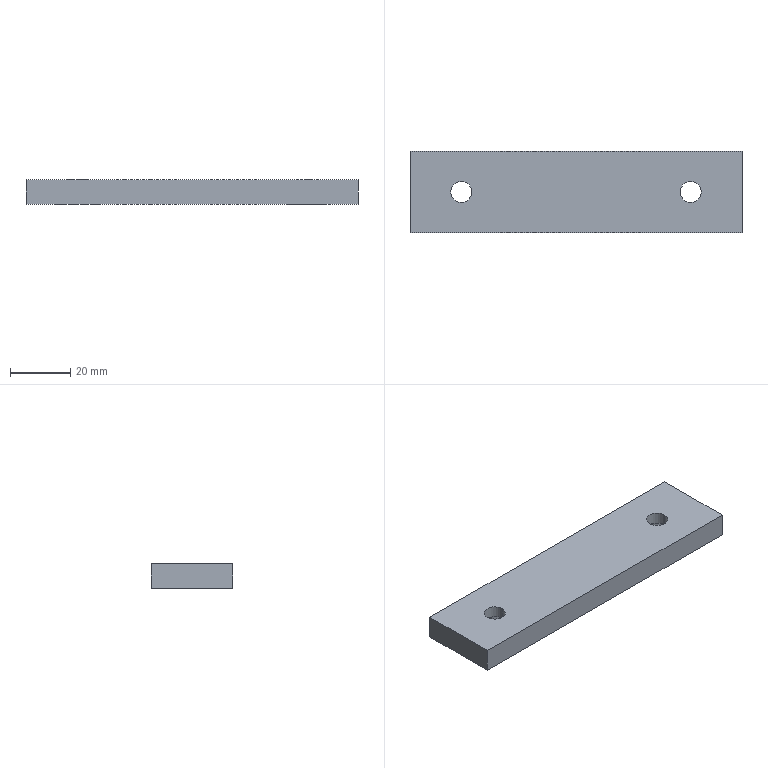Part | SolidWorks | features Extrusion 1, MirrorPattern 1, RevCut 1 | 1 solid | 14 faces | box 110 x 27 x 8 mm | volume 22658 mm3 | plane 6 | cylinder 4 | cone 4 | commonest cylinder face diameters 7 x4
STEP:
#1=CARTESIAN_POINT('',(41.5,0.,8.));
#2=VERTEX_POINT('',#1);
#3=CARTESIAN_POINT('',(34.5,0.,8.));
#4=VERTEX_POINT('',#3);
#5=CARTESIAN_POINT('',(38.,0.,8.));
#6=DIRECTION('',(0.,0.,1.));
#7=DIRECTION('',(1.,0.,0.));
#8=AXIS2_PLACEMENT_3D('',#5,#6,#7);
#9=CIRCLE('',#8,3.5);
#10=EDGE_CURVE('',#2,#4,#9,.T.);
#11=ORIENTED_EDGE('',*,*,#10,.T.);
#12=CARTESIAN_POINT('',(34.5,0.,4.));
#13=VERTEX_POINT('',#12);
#14=CARTESIAN_POINT('',(34.5,0.,0.));
#15=DIRECTION('',(0.,0.,-1.));
#16=VECTOR('',#15,1000.);
#17=LINE('',#14,#16);
#18=EDGE_CURVE('',#4,#13,#17,.T.);
#19=ORIENTED_EDGE('',*,*,#18,.T.);
#20=CARTESIAN_POINT('',(41.5,0.,4.));
#21=VERTEX_POINT('',#20);
#22=CARTESIAN_POINT('',(38.,0.,4.));
#23=DIRECTION('',(0.,0.,1.));
#24=DIRECTION('',(1.,0.,0.));
#25=AXIS2_PLACEMENT_3D('',#22,#23,#24);
#26=CIRCLE('',#25,3.5);
#27=EDGE_CURVE('',#21,#13,#26,.T.);
#28=ORIENTED_EDGE('',*,*,#27,.F.);
#29=CARTESIAN_POINT('',(41.5,0.,0.));
#30=DIRECTION('',(0.,0.,-1.));
#31=VECTOR('',#30,1000.);
#32=LINE('',#29,#31);
#33=EDGE_CURVE('',#2,#21,#32,.T.);
#34=ORIENTED_EDGE('',*,*,#33,.F.);
#35=EDGE_LOOP('',(#11,#19,#28,#34));
#36=FACE_OUTER_BOUND('',#35,.T.);
#37=CARTESIAN_POINT('',(38.,0.,0.));
#38=DIRECTION('',(0.,0.,-1.));
#39=DIRECTION('',(1.,0.,0.));
#40=AXIS2_PLACEMENT_3D('',#37,#38,#39);
#41=CYLINDRICAL_SURFACE('',#40,3.5);
#42=ADVANCED_FACE('',(#36),#41,.F.);
#43=ORIENTED_EDGE('',*,*,#27,.T.);
#44=CARTESIAN_POINT('',(30.5,0.,0.));
#45=VERTEX_POINT('',#44);
#46=CARTESIAN_POINT('',(34.5,0.,4.));
#47=DIRECTION('',(-0.7071,0.,-0.7071));
#48=VECTOR('',#47,1000.);
#49=LINE('',#46,#48);
#50=EDGE_CURVE('',#13,#45,#49,.T.);
#51=ORIENTED_EDGE('',*,*,#50,.T.);
#52=CARTESIAN_POINT('',(45.5,0.,0.));
#53=VERTEX_POINT('',#52);
#54=CARTESIAN_POINT('',(38.,0.,0.));
#55=DIRECTION('',(0.,0.,1.));
#56=DIRECTION('',(1.,0.,0.));
#57=AXIS2_PLACEMENT_3D('',#54,#55,#56);
#58=CIRCLE('',#57,7.5);
#59=EDGE_CURVE('',#53,#45,#58,.T.);
#60=ORIENTED_EDGE('',*,*,#59,.F.);
#61=CARTESIAN_POINT('',(41.5,0.,4.));
#62=DIRECTION('',(0.7071,0.,-0.7071));
#63=VECTOR('',#62,1000.);
#64=LINE('',#61,#63);
#65=EDGE_CURVE('',#21,#53,#64,.T.);
#66=ORIENTED_EDGE('',*,*,#65,.F.);
#67=EDGE_LOOP('',(#43,#51,#60,#66));
#68=FACE_OUTER_BOUND('',#67,.T.);
#69=CARTESIAN_POINT('',(38.,0.,4.));
#70=DIRECTION('',(0.,0.,-1.));
#71=DIRECTION('',(1.,0.,0.));
#72=AXIS2_PLACEMENT_3D('',#69,#70,#71);
#73=CONICAL_SURFACE('',#72,3.5,0.7854);
#74=ADVANCED_FACE('',(#68),#73,.F.);
#75=CARTESIAN_POINT('',(-34.5,0.,8.));
#76=VERTEX_POINT('',#75);
#77=CARTESIAN_POINT('',(-41.5,0.,8.));
#78=VERTEX_POINT('',#77);
#79=CARTESIAN_POINT('',(-38.,0.,8.));
#80=DIRECTION('',(0.,0.,-1.));
#81=DIRECTION('',(-1.,0.,0.));
#82=AXIS2_PLACEMENT_3D('',#79,#80,#81);
#83=CIRCLE('',#82,3.5);
#84=EDGE_CURVE('',#76,#78,#83,.T.);
#85=ORIENTED_EDGE('',*,*,#84,.F.);
#86=CARTESIAN_POINT('',(-34.5,0.,4.));
#87=VERTEX_POINT('',#86);
#88=CARTESIAN_POINT('',(-34.5,0.,0.));
#89=DIRECTION('',(0.,0.,-1.));
#90=VECTOR('',#89,1000.);
#91=LINE('',#88,#90);
#92=EDGE_CURVE('',#76,#87,#91,.T.);
#93=ORIENTED_EDGE('',*,*,#92,.T.);
#94=CARTESIAN_POINT('',(-41.5,0.,4.));
#95=VERTEX_POINT('',#94);
#96=CARTESIAN_POINT('',(-38.,0.,4.));
#97=DIRECTION('',(0.,0.,-1.));
#98=DIRECTION('',(-1.,0.,0.));
#99=AXIS2_PLACEMENT_3D('',#96,#97,#98);
#100=CIRCLE('',#99,3.5);
#101=EDGE_CURVE('',#87,#95,#100,.T.);
#102=ORIENTED_EDGE('',*,*,#101,.T.);
#103=CARTESIAN_POINT('',(-41.5,0.,0.));
#104=DIRECTION('',(0.,0.,-1.));
#105=VECTOR('',#104,1000.);
#106=LINE('',#103,#105);
#107=EDGE_CURVE('',#78,#95,#106,.T.);
#108=ORIENTED_EDGE('',*,*,#107,.F.);
#109=EDGE_LOOP('',(#85,#93,#102,#108));
#110=FACE_OUTER_BOUND('',#109,.T.);
#111=CARTESIAN_POINT('',(-38.,0.,0.));
#112=DIRECTION('',(0.,0.,-1.));
#113=DIRECTION('',(-1.,0.,0.));
#114=AXIS2_PLACEMENT_3D('',#111,#112,#113);
#115=CYLINDRICAL_SURFACE('',#114,3.5);
#116=ADVANCED_FACE('',(#110),#115,.F.);
#117=ORIENTED_EDGE('',*,*,#101,.F.);
#118=CARTESIAN_POINT('',(-30.5,0.,0.));
#119=VERTEX_POINT('',#118);
#120=CARTESIAN_POINT('',(-34.5,0.,4.));
#121=DIRECTION('',(0.7071,0.,-0.7071));
#122=VECTOR('',#121,1000.);
#123=LINE('',#120,#122);
#124=EDGE_CURVE('',#87,#119,#123,.T.);
#125=ORIENTED_EDGE('',*,*,#124,.T.);
#126=CARTESIAN_POINT('',(-45.5,0.,0.));
#127=VERTEX_POINT('',#126);
#128=CARTESIAN_POINT('',(-38.,0.,0.));
#129=DIRECTION('',(0.,0.,-1.));
#130=DIRECTION('',(-1.,0.,0.));
#131=AXIS2_PLACEMENT_3D('',#128,#129,#130);
#132=CIRCLE('',#131,7.5);
#133=EDGE_CURVE('',#119,#127,#132,.T.);
#134=ORIENTED_EDGE('',*,*,#133,.T.);
#135=CARTESIAN_POINT('',(-41.5,0.,4.));
#136=DIRECTION('',(-0.7071,0.,-0.7071));
#137=VECTOR('',#136,1000.);
#138=LINE('',#135,#137);
#139=EDGE_CURVE('',#95,#127,#138,.T.);
#140=ORIENTED_EDGE('',*,*,#139,.F.);
#141=EDGE_LOOP('',(#117,#125,#134,#140));
#142=FACE_OUTER_BOUND('',#141,.T.);
#143=CARTESIAN_POINT('',(-38.,0.,4.));
#144=DIRECTION('',(0.,0.,-1.));
#145=DIRECTION('',(-1.,0.,0.));
#146=AXIS2_PLACEMENT_3D('',#143,#144,#145);
#147=CONICAL_SURFACE('',#146,3.5,0.7854);
#148=ADVANCED_FACE('',(#142),#147,.F.);
#149=CARTESIAN_POINT('',(55.,-13.5,0.));
#150=VERTEX_POINT('',#149);
#151=CARTESIAN_POINT('',(55.,13.5,0.));
#152=VERTEX_POINT('',#151);
#153=CARTESIAN_POINT('',(55.,-13.5,0.));
#154=DIRECTION('',(0.,1.,0.));
#155=VECTOR('',#154,1000.);
#156=LINE('',#153,#155);
#157=EDGE_CURVE('',#150,#152,#156,.T.);
#158=ORIENTED_EDGE('',*,*,#157,.T.);
#159=CARTESIAN_POINT('',(55.,13.5,8.));
#160=VERTEX_POINT('',#159);
#161=CARTESIAN_POINT('',(55.,13.5,8.));
#162=DIRECTION('',(0.,0.,-1.));
#163=VECTOR('',#162,1000.);
#164=LINE('',#161,#163);
#165=EDGE_CURVE('',#160,#152,#164,.T.);
#166=ORIENTED_EDGE('',*,*,#165,.F.);
#167=CARTESIAN_POINT('',(55.,-13.5,8.));
#168=VERTEX_POINT('',#167);
#169=CARTESIAN_POINT('',(55.,-13.5,8.));
#170=DIRECTION('',(0.,1.,0.));
#171=VECTOR('',#170,1000.);
#172=LINE('',#169,#171);
#173=EDGE_CURVE('',#168,#160,#172,.T.);
#174=ORIENTED_EDGE('',*,*,#173,.F.);
#175=CARTESIAN_POINT('',(55.,-13.5,8.));
#176=DIRECTION('',(0.,0.,-1.));
#177=VECTOR('',#176,1000.);
#178=LINE('',#175,#177);
#179=EDGE_CURVE('',#168,#150,#178,.T.);
#180=ORIENTED_EDGE('',*,*,#179,.T.);
#181=EDGE_LOOP('',(#158,#166,#174,#180));
#182=FACE_OUTER_BOUND('',#181,.T.);
#183=CARTESIAN_POINT('',(55.,-13.5,8.));
#184=DIRECTION('',(-1.,0.,0.));
#185=DIRECTION('',(0.,0.,1.));
#186=AXIS2_PLACEMENT_3D('',#183,#184,#185);
#187=PLANE('',#186);
#188=ADVANCED_FACE('',(#182),#187,.F.);
#189=CARTESIAN_POINT('',(-55.,13.5,0.));
#190=VERTEX_POINT('',#189);
#191=CARTESIAN_POINT('',(-55.,13.5,0.));
#192=DIRECTION('',(-1.,0.,0.));
#193=VECTOR('',#192,1000.);
#194=LINE('',#191,#193);
#195=EDGE_CURVE('',#152,#190,#194,.T.);
#196=ORIENTED_EDGE('',*,*,#195,.T.);
#197=CARTESIAN_POINT('',(-55.,13.5,8.));
#198=VERTEX_POINT('',#197);
#199=CARTESIAN_POINT('',(-55.,13.5,8.));
#200=DIRECTION('',(0.,0.,-1.));
#201=VECTOR('',#200,1000.);
#202=LINE('',#199,#201);
#203=EDGE_CURVE('',#198,#190,#202,.T.);
#204=ORIENTED_EDGE('',*,*,#203,.F.);
#205=CARTESIAN_POINT('',(-55.,13.5,8.));
#206=DIRECTION('',(-1.,0.,0.));
#207=VECTOR('',#206,1000.);
#208=LINE('',#205,#207);
#209=EDGE_CURVE('',#160,#198,#208,.T.);
#210=ORIENTED_EDGE('',*,*,#209,.F.);
#211=ORIENTED_EDGE('',*,*,#165,.T.);
#212=EDGE_LOOP('',(#196,#204,#210,#211));
#213=FACE_OUTER_BOUND('',#212,.T.);
#214=CARTESIAN_POINT('',(-55.,13.5,8.));
#215=DIRECTION('',(0.,-1.,0.));
#216=DIRECTION('',(0.,0.,-1.));
#217=AXIS2_PLACEMENT_3D('',#214,#215,#216);
#218=PLANE('',#217);
#219=ADVANCED_FACE('',(#213),#218,.F.);
#220=CARTESIAN_POINT('',(-55.,-13.5,0.));
#221=VERTEX_POINT('',#220);
#222=CARTESIAN_POINT('',(-55.,-13.5,0.));
#223=DIRECTION('',(0.,-1.,0.));
#224=VECTOR('',#223,1000.);
#225=LINE('',#222,#224);
#226=EDGE_CURVE('',#190,#221,#225,.T.);
#227=ORIENTED_EDGE('',*,*,#226,.T.);
#228=CARTESIAN_POINT('',(-55.,-13.5,8.));
#229=VERTEX_POINT('',#228);
#230=CARTESIAN_POINT('',(-55.,-13.5,8.));
#231=DIRECTION('',(0.,0.,-1.));
#232=VECTOR('',#231,1000.);
#233=LINE('',#230,#232);
#234=EDGE_CURVE('',#229,#221,#233,.T.);
#235=ORIENTED_EDGE('',*,*,#234,.F.);
#236=CARTESIAN_POINT('',(-55.,-13.5,8.));
#237=DIRECTION('',(0.,-1.,0.));
#238=VECTOR('',#237,1000.);
#239=LINE('',#236,#238);
#240=EDGE_CURVE('',#198,#229,#239,.T.);
#241=ORIENTED_EDGE('',*,*,#240,.F.);
#242=ORIENTED_EDGE('',*,*,#203,.T.);
#243=EDGE_LOOP('',(#227,#235,#241,#242));
#244=FACE_OUTER_BOUND('',#243,.T.);
#245=CARTESIAN_POINT('',(-55.,-13.5,8.));
#246=DIRECTION('',(1.,0.,0.));
#247=DIRECTION('',(0.,0.,-1.));
#248=AXIS2_PLACEMENT_3D('',#245,#246,#247);
#249=PLANE('',#248);
#250=ADVANCED_FACE('',(#244),#249,.F.);
#251=CARTESIAN_POINT('',(-55.,-13.5,0.));
#252=DIRECTION('',(1.,0.,0.));
#253=VECTOR('',#252,1000.);
#254=LINE('',#251,#253);
#255=EDGE_CURVE('',#221,#150,#254,.T.);
#256=ORIENTED_EDGE('',*,*,#255,.T.);
#257=ORIENTED_EDGE('',*,*,#179,.F.);
#258=CARTESIAN_POINT('',(-55.,-13.5,8.));
#259=DIRECTION('',(1.,0.,0.));
#260=VECTOR('',#259,1000.);
#261=LINE('',#258,#260);
#262=EDGE_CURVE('',#229,#168,#261,.T.);
#263=ORIENTED_EDGE('',*,*,#262,.F.);
#264=ORIENTED_EDGE('',*,*,#234,.T.);
#265=EDGE_LOOP('',(#256,#257,#263,#264));
#266=FACE_OUTER_BOUND('',#265,.T.);
#267=CARTESIAN_POINT('',(-55.,-13.5,8.));
#268=DIRECTION('',(0.,1.,0.));
#269=DIRECTION('',(0.,0.,1.));
#270=AXIS2_PLACEMENT_3D('',#267,#268,#269);
#271=PLANE('',#270);
#272=ADVANCED_FACE('',(#266),#271,.F.);
#273=ORIENTED_EDGE('',*,*,#10,.F.);
#274=CARTESIAN_POINT('',(38.,0.,8.));
#275=DIRECTION('',(0.,0.,1.));
#276=DIRECTION('',(1.,0.,0.));
#277=AXIS2_PLACEMENT_3D('',#274,#275,#276);
#278=CIRCLE('',#277,3.5);
#279=EDGE_CURVE('',#4,#2,#278,.T.);
#280=ORIENTED_EDGE('',*,*,#279,.F.);
#281=EDGE_LOOP('',(#273,#280));
#282=FACE_BOUND('',#281,.T.);
#283=CARTESIAN_POINT('',(-38.,0.,8.));
#284=DIRECTION('',(0.,0.,-1.));
#285=DIRECTION('',(-1.,0.,0.));
#286=AXIS2_PLACEMENT_3D('',#283,#284,#285);
#287=CIRCLE('',#286,3.5);
#288=EDGE_CURVE('',#78,#76,#287,.T.);
#289=ORIENTED_EDGE('',*,*,#288,.T.);
#290=ORIENTED_EDGE('',*,*,#84,.T.);
#291=EDGE_LOOP('',(#289,#290));
#292=FACE_BOUND('',#291,.T.);
#293=ORIENTED_EDGE('',*,*,#173,.T.);
#294=ORIENTED_EDGE('',*,*,#209,.T.);
#295=ORIENTED_EDGE('',*,*,#240,.T.);
#296=ORIENTED_EDGE('',*,*,#262,.T.);
#297=EDGE_LOOP('',(#293,#294,#295,#296));
#298=FACE_OUTER_BOUND('',#297,.T.);
#299=CARTESIAN_POINT('',(0.,0.,8.));
#300=DIRECTION('',(0.,0.,-1.));
#301=DIRECTION('',(-1.,0.,0.));
#302=AXIS2_PLACEMENT_3D('',#299,#300,#301);
#303=PLANE('',#302);
#304=ADVANCED_FACE('',(#282,#292,#298),#303,.F.);
#305=ORIENTED_EDGE('',*,*,#59,.T.);
#306=CARTESIAN_POINT('',(38.,0.,0.));
#307=DIRECTION('',(0.,0.,1.));
#308=DIRECTION('',(1.,0.,0.));
#309=AXIS2_PLACEMENT_3D('',#306,#307,#308);
#310=CIRCLE('',#309,7.5);
#311=EDGE_CURVE('',#45,#53,#310,.T.);
#312=ORIENTED_EDGE('',*,*,#311,.T.);
#313=EDGE_LOOP('',(#305,#312));
#314=FACE_BOUND('',#313,.T.);
#315=CARTESIAN_POINT('',(-38.,0.,0.));
#316=DIRECTION('',(0.,0.,-1.));
#317=DIRECTION('',(-1.,0.,0.));
#318=AXIS2_PLACEMENT_3D('',#315,#316,#317);
#319=CIRCLE('',#318,7.5);
#320=EDGE_CURVE('',#127,#119,#319,.T.);
#321=ORIENTED_EDGE('',*,*,#320,.F.);
#322=ORIENTED_EDGE('',*,*,#133,.F.);
#323=EDGE_LOOP('',(#321,#322));
#324=FACE_BOUND('',#323,.T.);
#325=ORIENTED_EDGE('',*,*,#157,.F.);
#326=ORIENTED_EDGE('',*,*,#255,.F.);
#327=ORIENTED_EDGE('',*,*,#226,.F.);
#328=ORIENTED_EDGE('',*,*,#195,.F.);
#329=EDGE_LOOP('',(#325,#326,#327,#328));
#330=FACE_OUTER_BOUND('',#329,.T.);
#331=CARTESIAN_POINT('',(0.,0.,0.));
#332=DIRECTION('',(0.,0.,-1.));
#333=DIRECTION('',(-1.,0.,0.));
#334=AXIS2_PLACEMENT_3D('',#331,#332,#333);
#335=PLANE('',#334);
#336=ADVANCED_FACE('',(#314,#324,#330),#335,.T.);
#337=ORIENTED_EDGE('',*,*,#124,.F.);
#338=CARTESIAN_POINT('',(-38.,0.,4.));
#339=DIRECTION('',(0.,0.,-1.));
#340=DIRECTION('',(-1.,0.,0.));
#341=AXIS2_PLACEMENT_3D('',#338,#339,#340);
#342=CIRCLE('',#341,3.5);
#343=EDGE_CURVE('',#95,#87,#342,.T.);
#344=ORIENTED_EDGE('',*,*,#343,.F.);
#345=ORIENTED_EDGE('',*,*,#139,.T.);
#346=ORIENTED_EDGE('',*,*,#320,.T.);
#347=EDGE_LOOP('',(#337,#344,#345,#346));
#348=FACE_OUTER_BOUND('',#347,.T.);
#349=CARTESIAN_POINT('',(-38.,0.,4.));
#350=DIRECTION('',(0.,0.,-1.));
#351=DIRECTION('',(-1.,0.,0.));
#352=AXIS2_PLACEMENT_3D('',#349,#350,#351);
#353=CONICAL_SURFACE('',#352,3.5,0.7854);
#354=ADVANCED_FACE('',(#348),#353,.F.);
#355=ORIENTED_EDGE('',*,*,#92,.F.);
#356=ORIENTED_EDGE('',*,*,#288,.F.);
#357=ORIENTED_EDGE('',*,*,#107,.T.);
#358=ORIENTED_EDGE('',*,*,#343,.T.);
#359=EDGE_LOOP('',(#355,#356,#357,#358));
#360=FACE_OUTER_BOUND('',#359,.T.);
#361=CARTESIAN_POINT('',(-38.,0.,0.));
#362=DIRECTION('',(0.,0.,-1.));
#363=DIRECTION('',(-1.,0.,0.));
#364=AXIS2_PLACEMENT_3D('',#361,#362,#363);
#365=CYLINDRICAL_SURFACE('',#364,3.5);
#366=ADVANCED_FACE('',(#360),#365,.F.);
#367=ORIENTED_EDGE('',*,*,#50,.F.);
#368=CARTESIAN_POINT('',(38.,0.,4.));
#369=DIRECTION('',(0.,0.,1.));
#370=DIRECTION('',(1.,0.,0.));
#371=AXIS2_PLACEMENT_3D('',#368,#369,#370);
#372=CIRCLE('',#371,3.5);
#373=EDGE_CURVE('',#13,#21,#372,.T.);
#374=ORIENTED_EDGE('',*,*,#373,.T.);
#375=ORIENTED_EDGE('',*,*,#65,.T.);
#376=ORIENTED_EDGE('',*,*,#311,.F.);
#377=EDGE_LOOP('',(#367,#374,#375,#376));
#378=FACE_OUTER_BOUND('',#377,.T.);
#379=CARTESIAN_POINT('',(38.,0.,4.));
#380=DIRECTION('',(0.,0.,-1.));
#381=DIRECTION('',(1.,0.,0.));
#382=AXIS2_PLACEMENT_3D('',#379,#380,#381);
#383=CONICAL_SURFACE('',#382,3.5,0.7854);
#384=ADVANCED_FACE('',(#378),#383,.F.);
#385=ORIENTED_EDGE('',*,*,#18,.F.);
#386=ORIENTED_EDGE('',*,*,#279,.T.);
#387=ORIENTED_EDGE('',*,*,#33,.T.);
#388=ORIENTED_EDGE('',*,*,#373,.F.);
#389=EDGE_LOOP('',(#385,#386,#387,#388));
#390=FACE_OUTER_BOUND('',#389,.T.);
#391=CARTESIAN_POINT('',(38.,0.,0.));
#392=DIRECTION('',(0.,0.,-1.));
#393=DIRECTION('',(1.,0.,0.));
#394=AXIS2_PLACEMENT_3D('',#391,#392,#393);
#395=CYLINDRICAL_SURFACE('',#394,3.5);
#396=ADVANCED_FACE('',(#390),#395,.F.);
#397=CLOSED_SHELL('',(#42,#74,#116,#148,#188,#219,#250,#272,#304,#336,#354,#366,#384,#396));
#398=MANIFOLD_SOLID_BREP('',#397);
#399=CARTESIAN_POINT('',(0.,0.,0.));
#400=DIRECTION('',(0.,0.,1.));
#401=DIRECTION('',(1.,0.,0.));
#402=AXIS2_PLACEMENT_3D('',#399,#400,#401);
#403=(LENGTH_UNIT()NAMED_UNIT(*)SI_UNIT(.MILLI.,.METRE.));
#404=UNCERTAINTY_MEASURE_WITH_UNIT(LENGTH_MEASURE(0.00001),#403,'','');
#405=(NAMED_UNIT(*)PLANE_ANGLE_UNIT()SI_UNIT($,.RADIAN.));
#406=(NAMED_UNIT(*)SI_UNIT($,.STERADIAN.)SOLID_ANGLE_UNIT());
#407=(GEOMETRIC_REPRESENTATION_CONTEXT(3)GLOBAL_UNCERTAINTY_ASSIGNED_CONTEXT((#404))GLOBAL_UNIT_ASSIGNED_CONTEXT((#403,#405,#406))REPRESENTATION_CONTEXT('',''));
#408=ADVANCED_BREP_SHAPE_REPRESENTATION('',(#398,#402),#407);